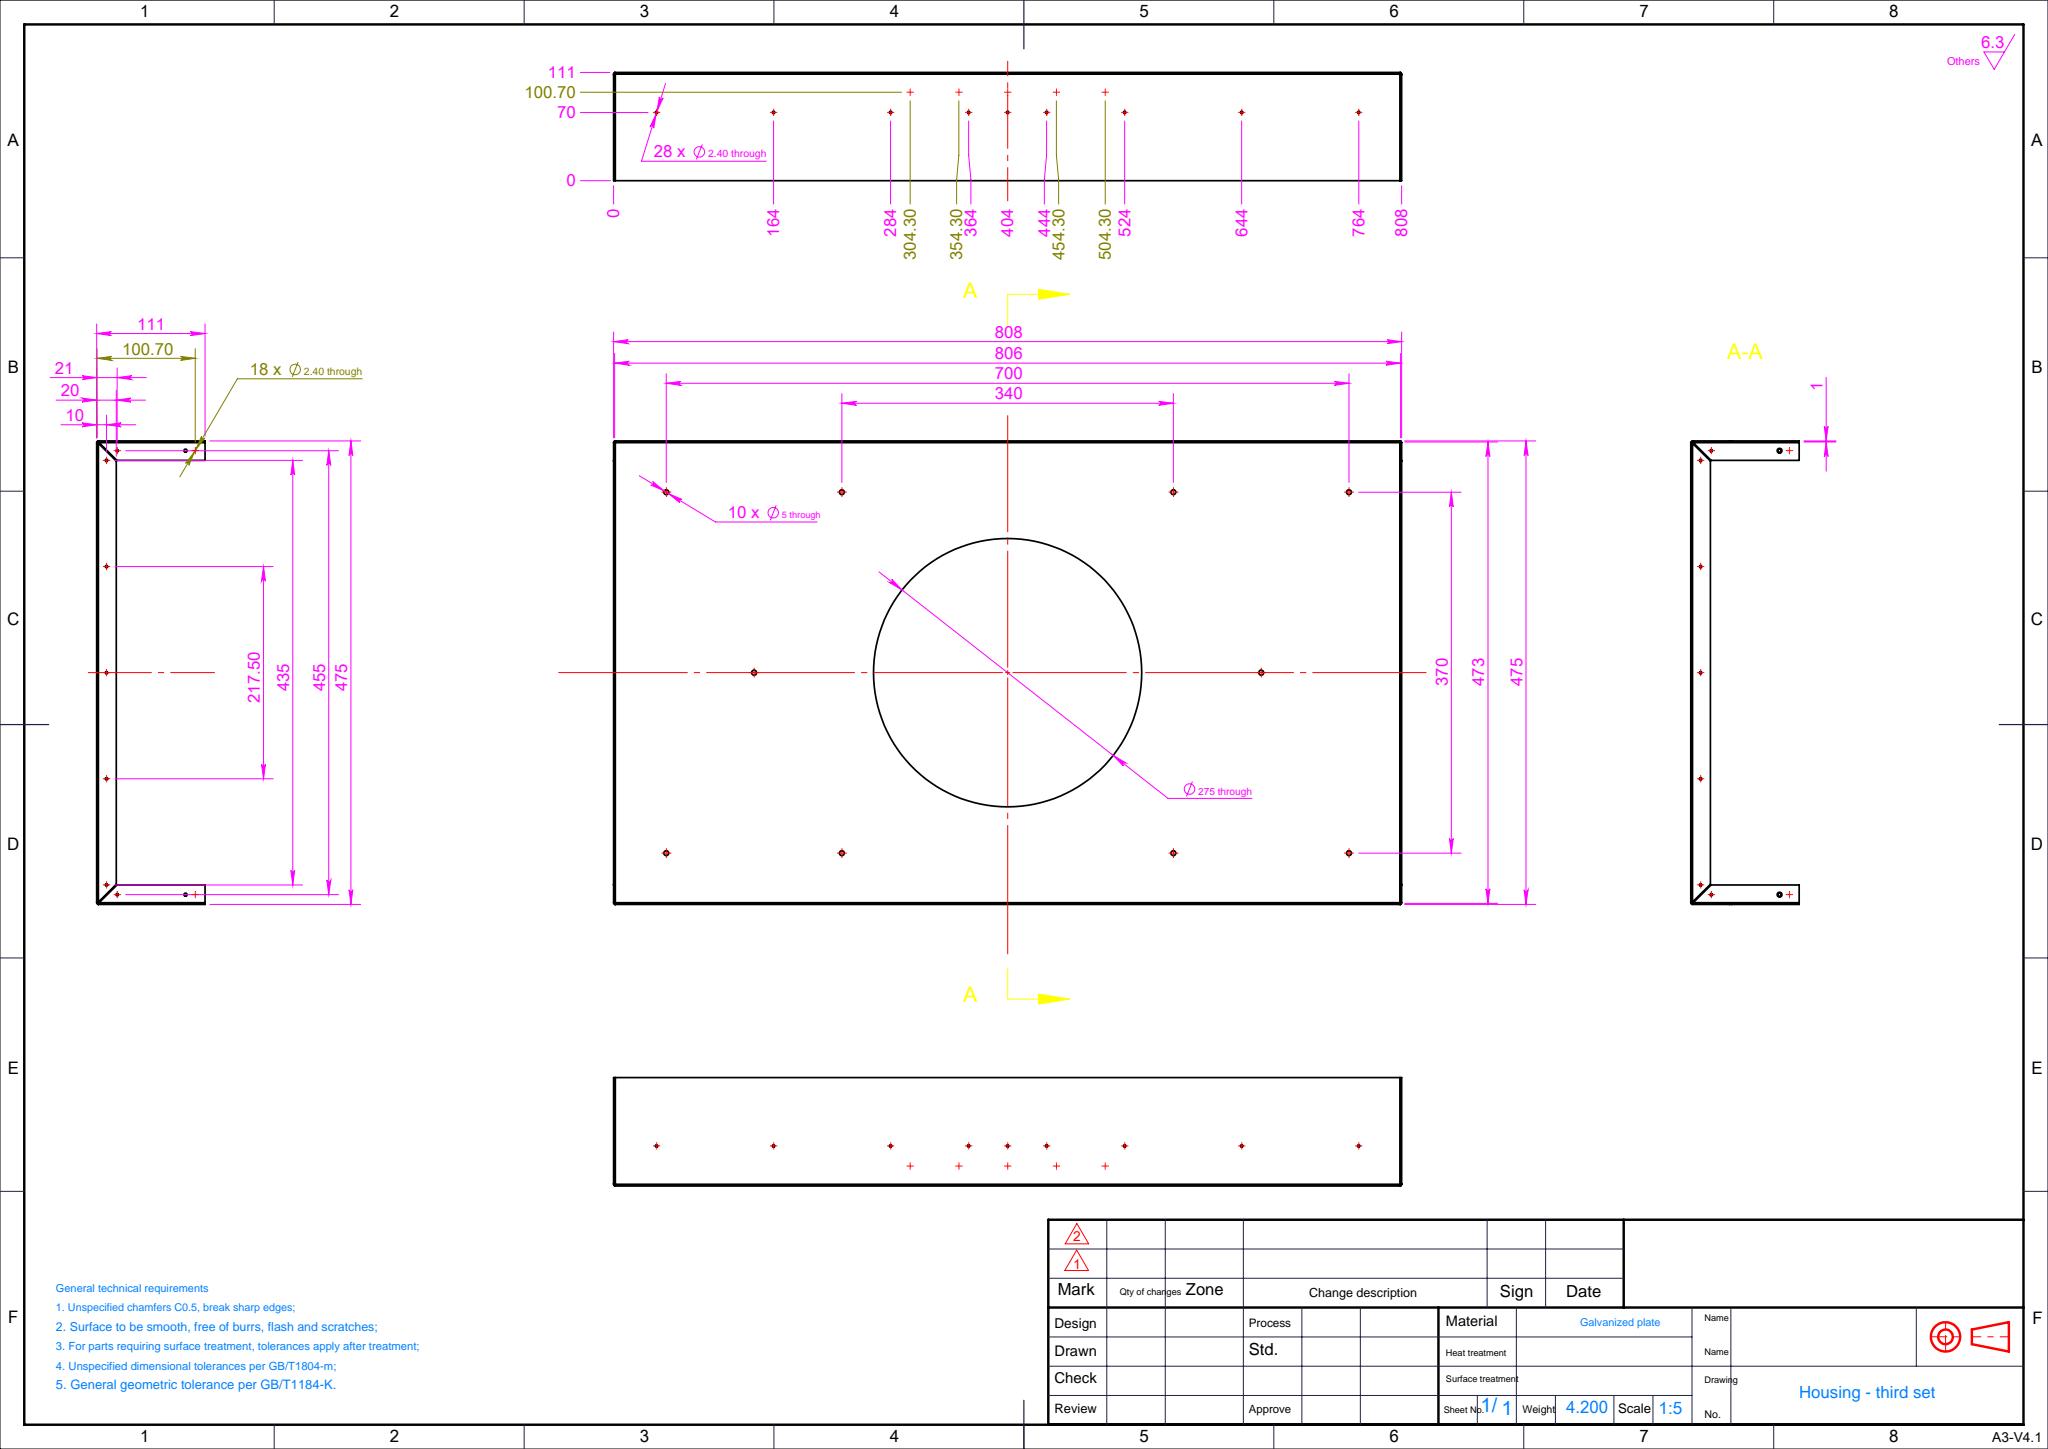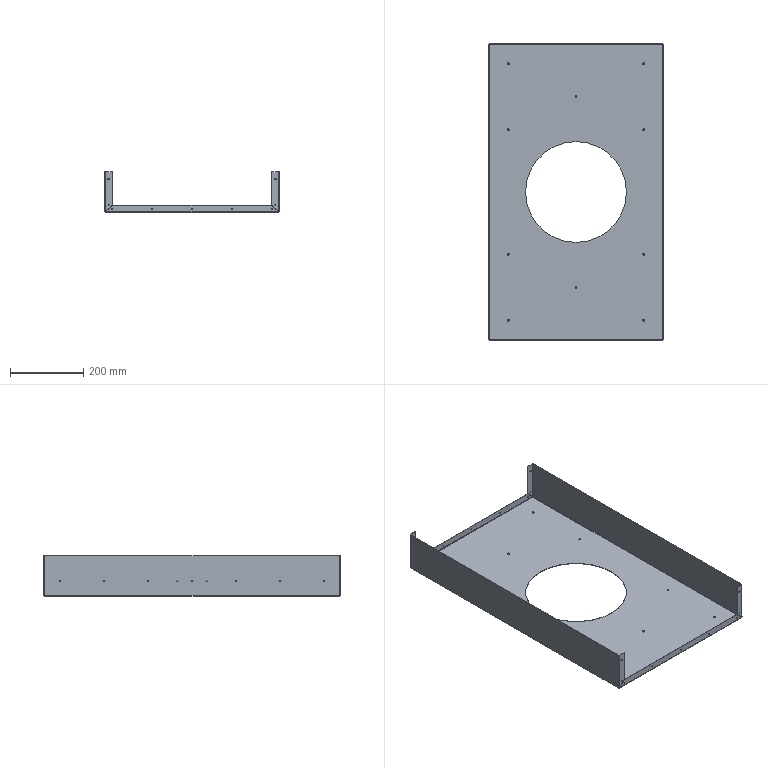Part | SolidWorks | features 3DProfileFeature 5, HoleWzd 5, SketchPattern 4, Chamfer 3, EdgeFlange 2, ICE 2, FlatPattern 1, SMBaseFlange 1, SheetMetal 1 | 1 solid | 180 faces | box 475 x 808 x 111 mm | volume 524962 mm3 | cylinder 110 | plane 54 | cone 8 | spline 8 | commonest cylinder face diameters 2.4 x64 5 x20 1.473 x8 3.2 x8 3.473 x8 275 x2